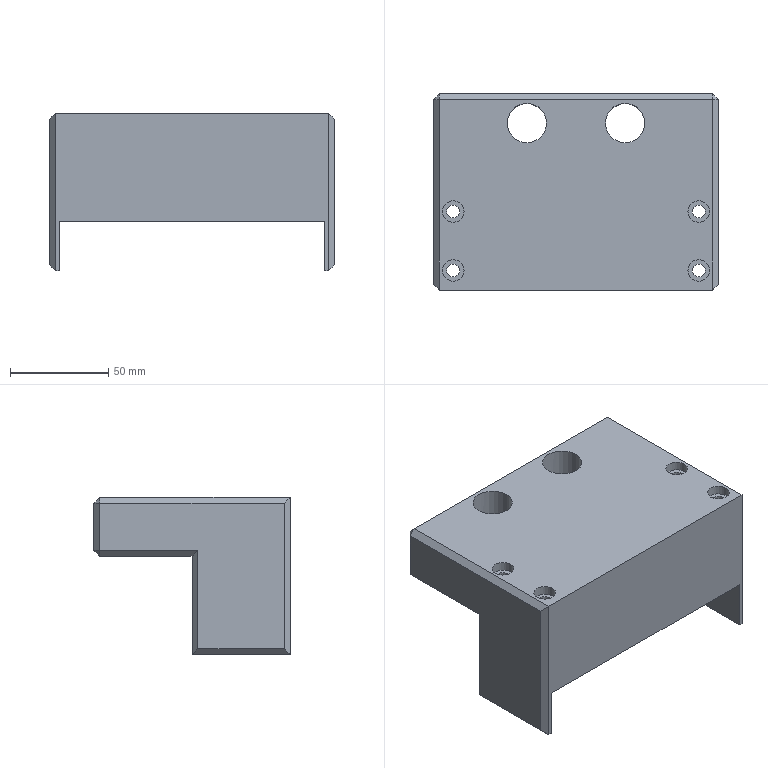Part | 1 solid | 48 faces | box 145 x 100 x 80 mm | volume 596395 mm3 | plane 34 | cylinder 12 | cone 2 | commonest cylinder face diameters 6.6 x4 11 x4 5 x2 20 x2
STEP:
#1=CARTESIAN_POINT('',(72.5,-47.,-3.));
#2=VERTEX_POINT('',#1);
#3=CARTESIAN_POINT('',(72.5,-47.,-77.));
#4=VERTEX_POINT('',#3);
#5=CARTESIAN_POINT('',(72.5,-47.,0.));
#6=DIRECTION('',(0.,0.,-1.));
#7=VECTOR('',#6,1000.);
#8=LINE('',#5,#7);
#9=EDGE_CURVE('',#2,#4,#8,.T.);
#10=ORIENTED_EDGE('',*,*,#9,.T.);
#11=CARTESIAN_POINT('',(72.5,-3.,-77.));
#12=VERTEX_POINT('',#11);
#13=CARTESIAN_POINT('',(72.5,50.,-77.));
#14=DIRECTION('',(0.,1.,0.));
#15=VECTOR('',#14,1000.);
#16=LINE('',#13,#15);
#17=EDGE_CURVE('',#4,#12,#16,.T.);
#18=ORIENTED_EDGE('',*,*,#17,.T.);
#19=CARTESIAN_POINT('',(72.5,-3.,-27.));
#20=VERTEX_POINT('',#19);
#21=CARTESIAN_POINT('',(72.5,-3.,0.));
#22=DIRECTION('',(0.,0.,1.));
#23=VECTOR('',#22,1000.);
#24=LINE('',#21,#23);
#25=EDGE_CURVE('',#12,#20,#24,.T.);
#26=ORIENTED_EDGE('',*,*,#25,.T.);
#27=CARTESIAN_POINT('',(72.5,47.,-27.));
#28=VERTEX_POINT('',#27);
#29=CARTESIAN_POINT('',(72.5,50.,-27.));
#30=DIRECTION('',(0.,1.,0.));
#31=VECTOR('',#30,1000.);
#32=LINE('',#29,#31);
#33=EDGE_CURVE('',#20,#28,#32,.T.);
#34=ORIENTED_EDGE('',*,*,#33,.T.);
#35=CARTESIAN_POINT('',(72.5,47.,-3.));
#36=VERTEX_POINT('',#35);
#37=CARTESIAN_POINT('',(72.5,47.,0.));
#38=DIRECTION('',(0.,0.,1.));
#39=VECTOR('',#38,1000.);
#40=LINE('',#37,#39);
#41=EDGE_CURVE('',#28,#36,#40,.T.);
#42=ORIENTED_EDGE('',*,*,#41,.T.);
#43=CARTESIAN_POINT('',(72.5,-50.,-3.));
#44=DIRECTION('',(0.,-1.,0.));
#45=VECTOR('',#44,1000.);
#46=LINE('',#43,#45);
#47=EDGE_CURVE('',#36,#2,#46,.T.);
#48=ORIENTED_EDGE('',*,*,#47,.T.);
#49=EDGE_LOOP('',(#10,#18,#26,#34,#42,#48));
#50=FACE_BOUND('',#49,.T.);
#51=CARTESIAN_POINT('',(72.5,50.,0.));
#52=DIRECTION('',(-1.,0.,0.));
#53=DIRECTION('',(0.,0.,1.));
#54=AXIS2_PLACEMENT_3D('',#51,#52,#53);
#55=PLANE('',#54);
#56=ADVANCED_FACE('',(#50),#55,.F.);
#57=CARTESIAN_POINT('',(67.5,0.,-80.));
#58=VERTEX_POINT('',#57);
#59=CARTESIAN_POINT('',(69.5,0.,-80.));
#60=VERTEX_POINT('',#59);
#61=CARTESIAN_POINT('',(-72.5,0.,-80.));
#62=DIRECTION('',(1.,0.,0.));
#63=VECTOR('',#62,1000.);
#64=LINE('',#61,#63);
#65=EDGE_CURVE('',#58,#60,#64,.T.);
#66=ORIENTED_EDGE('',*,*,#65,.T.);
#67=CARTESIAN_POINT('',(69.5,-50.,-80.));
#68=VERTEX_POINT('',#67);
#69=CARTESIAN_POINT('',(69.5,50.,-80.));
#70=DIRECTION('',(0.,-1.,0.));
#71=VECTOR('',#70,1000.);
#72=LINE('',#69,#71);
#73=EDGE_CURVE('',#60,#68,#72,.T.);
#74=ORIENTED_EDGE('',*,*,#73,.T.);
#75=CARTESIAN_POINT('',(67.5,-50.,-80.));
#76=VERTEX_POINT('',#75);
#77=CARTESIAN_POINT('',(72.5,-50.,-80.));
#78=DIRECTION('',(-1.,0.,0.));
#79=VECTOR('',#78,1000.);
#80=LINE('',#77,#79);
#81=EDGE_CURVE('',#68,#76,#80,.T.);
#82=ORIENTED_EDGE('',*,*,#81,.T.);
#83=CARTESIAN_POINT('',(67.5,50.,-80.));
#84=DIRECTION('',(0.,-1.,0.));
#85=VECTOR('',#84,1000.);
#86=LINE('',#83,#85);
#87=EDGE_CURVE('',#58,#76,#86,.T.);
#88=ORIENTED_EDGE('',*,*,#87,.F.);
#89=EDGE_LOOP('',(#66,#74,#82,#88));
#90=FACE_BOUND('',#89,.T.);
#91=CARTESIAN_POINT('',(72.5,50.,-80.));
#92=DIRECTION('',(0.,0.,1.));
#93=DIRECTION('',(1.,0.,0.));
#94=AXIS2_PLACEMENT_3D('',#91,#92,#93);
#95=PLANE('',#94);
#96=ADVANCED_FACE('',(#90),#95,.F.);
#97=CARTESIAN_POINT('',(67.5,0.,-55.));
#98=VERTEX_POINT('',#97);
#99=CARTESIAN_POINT('',(67.5,-50.,-55.));
#100=VERTEX_POINT('',#99);
#101=CARTESIAN_POINT('',(67.5,50.,-55.));
#102=DIRECTION('',(0.,-1.,0.));
#103=VECTOR('',#102,1000.);
#104=LINE('',#101,#103);
#105=EDGE_CURVE('',#98,#100,#104,.T.);
#106=ORIENTED_EDGE('',*,*,#105,.F.);
#107=CARTESIAN_POINT('',(67.5,0.,-80.));
#108=DIRECTION('',(0.,0.,-1.));
#109=VECTOR('',#108,1000.);
#110=LINE('',#107,#109);
#111=EDGE_CURVE('',#98,#58,#110,.T.);
#112=ORIENTED_EDGE('',*,*,#111,.T.);
#113=ORIENTED_EDGE('',*,*,#87,.T.);
#114=CARTESIAN_POINT('',(67.5,-50.,-80.));
#115=DIRECTION('',(0.,0.,1.));
#116=VECTOR('',#115,1000.);
#117=LINE('',#114,#116);
#118=EDGE_CURVE('',#76,#100,#117,.T.);
#119=ORIENTED_EDGE('',*,*,#118,.T.);
#120=EDGE_LOOP('',(#106,#112,#113,#119));
#121=FACE_BOUND('',#120,.T.);
#122=CARTESIAN_POINT('',(67.5,50.,-80.));
#123=DIRECTION('',(1.,0.,0.));
#124=DIRECTION('',(0.,0.,-1.));
#125=AXIS2_PLACEMENT_3D('',#122,#123,#124);
#126=PLANE('',#125);
#127=ADVANCED_FACE('',(#121),#126,.F.);
#128=CARTESIAN_POINT('',(-65.8,-10.,-55.));
#129=VERTEX_POINT('',#128);
#130=CARTESIAN_POINT('',(-62.5,-10.,-55.));
#131=DIRECTION('',(0.,0.,-1.));
#132=DIRECTION('',(-1.,0.,0.));
#133=AXIS2_PLACEMENT_3D('',#130,#131,#132);
#134=CIRCLE('',#133,3.3);
#135=EDGE_CURVE('',#129,#129,#134,.T.);
#136=ORIENTED_EDGE('',*,*,#135,.F.);
#137=EDGE_LOOP('',(#136));
#138=FACE_BOUND('',#137,.T.);
#139=CARTESIAN_POINT('',(-65.8,-40.,-55.));
#140=VERTEX_POINT('',#139);
#141=CARTESIAN_POINT('',(-62.5,-40.,-55.));
#142=DIRECTION('',(0.,0.,-1.));
#143=DIRECTION('',(-1.,0.,0.));
#144=AXIS2_PLACEMENT_3D('',#141,#142,#143);
#145=CIRCLE('',#144,3.3);
#146=EDGE_CURVE('',#140,#140,#145,.T.);
#147=ORIENTED_EDGE('',*,*,#146,.F.);
#148=EDGE_LOOP('',(#147));
#149=FACE_BOUND('',#148,.T.);
#150=CARTESIAN_POINT('',(59.2,-10.,-55.));
#151=VERTEX_POINT('',#150);
#152=CARTESIAN_POINT('',(62.5,-10.,-55.));
#153=DIRECTION('',(0.,0.,-1.));
#154=DIRECTION('',(-1.,0.,0.));
#155=AXIS2_PLACEMENT_3D('',#152,#153,#154);
#156=CIRCLE('',#155,3.3);
#157=EDGE_CURVE('',#151,#151,#156,.T.);
#158=ORIENTED_EDGE('',*,*,#157,.F.);
#159=EDGE_LOOP('',(#158));
#160=FACE_BOUND('',#159,.T.);
#161=CARTESIAN_POINT('',(59.2,-40.,-55.));
#162=VERTEX_POINT('',#161);
#163=CARTESIAN_POINT('',(62.5,-40.,-55.));
#164=DIRECTION('',(0.,0.,-1.));
#165=DIRECTION('',(-1.,0.,0.));
#166=AXIS2_PLACEMENT_3D('',#163,#164,#165);
#167=CIRCLE('',#166,3.3);
#168=EDGE_CURVE('',#162,#162,#167,.T.);
#169=ORIENTED_EDGE('',*,*,#168,.F.);
#170=EDGE_LOOP('',(#169));
#171=FACE_BOUND('',#170,.T.);
#172=CARTESIAN_POINT('',(-67.5,0.,-55.));
#173=VERTEX_POINT('',#172);
#174=CARTESIAN_POINT('',(-67.5,0.,-55.));
#175=DIRECTION('',(-1.,0.,0.));
#176=VECTOR('',#175,1000.);
#177=LINE('',#174,#176);
#178=EDGE_CURVE('',#98,#173,#177,.T.);
#179=ORIENTED_EDGE('',*,*,#178,.F.);
#180=ORIENTED_EDGE('',*,*,#105,.T.);
#181=CARTESIAN_POINT('',(-67.5,-50.,-55.));
#182=VERTEX_POINT('',#181);
#183=CARTESIAN_POINT('',(-67.5,-50.,-55.));
#184=DIRECTION('',(1.,0.,0.));
#185=VECTOR('',#184,1000.);
#186=LINE('',#183,#185);
#187=EDGE_CURVE('',#182,#100,#186,.T.);
#188=ORIENTED_EDGE('',*,*,#187,.F.);
#189=CARTESIAN_POINT('',(-67.5,50.,-55.));
#190=DIRECTION('',(0.,-1.,0.));
#191=VECTOR('',#190,1000.);
#192=LINE('',#189,#191);
#193=EDGE_CURVE('',#173,#182,#192,.T.);
#194=ORIENTED_EDGE('',*,*,#193,.F.);
#195=EDGE_LOOP('',(#179,#180,#188,#194));
#196=FACE_BOUND('',#195,.T.);
#197=CARTESIAN_POINT('',(-67.5,50.,-55.));
#198=DIRECTION('',(0.,0.,-1.));
#199=DIRECTION('',(-1.,0.,0.));
#200=AXIS2_PLACEMENT_3D('',#197,#198,#199);
#201=PLANE('',#200);
#202=ADVANCED_FACE('',(#138,#149,#160,#171,#196),#201,.T.);
#203=CARTESIAN_POINT('',(-67.5,0.,-80.));
#204=VERTEX_POINT('',#203);
#205=CARTESIAN_POINT('',(-67.5,0.,-80.));
#206=DIRECTION('',(0.,0.,-1.));
#207=VECTOR('',#206,1000.);
#208=LINE('',#205,#207);
#209=EDGE_CURVE('',#173,#204,#208,.T.);
#210=ORIENTED_EDGE('',*,*,#209,.F.);
#211=ORIENTED_EDGE('',*,*,#193,.T.);
#212=CARTESIAN_POINT('',(-67.5,-50.,-80.));
#213=VERTEX_POINT('',#212);
#214=CARTESIAN_POINT('',(-67.5,-50.,-80.));
#215=DIRECTION('',(0.,0.,1.));
#216=VECTOR('',#215,1000.);
#217=LINE('',#214,#216);
#218=EDGE_CURVE('',#213,#182,#217,.T.);
#219=ORIENTED_EDGE('',*,*,#218,.F.);
#220=CARTESIAN_POINT('',(-67.5,50.,-80.));
#221=DIRECTION('',(0.,-1.,0.));
#222=VECTOR('',#221,1000.);
#223=LINE('',#220,#222);
#224=EDGE_CURVE('',#204,#213,#223,.T.);
#225=ORIENTED_EDGE('',*,*,#224,.F.);
#226=EDGE_LOOP('',(#210,#211,#219,#225));
#227=FACE_BOUND('',#226,.T.);
#228=CARTESIAN_POINT('',(-67.5,50.,-80.));
#229=DIRECTION('',(1.,0.,0.));
#230=DIRECTION('',(0.,0.,-1.));
#231=AXIS2_PLACEMENT_3D('',#228,#229,#230);
#232=PLANE('',#231);
#233=ADVANCED_FACE('',(#227),#232,.T.);
#234=CARTESIAN_POINT('',(-69.5,-50.,-80.));
#235=VERTEX_POINT('',#234);
#236=CARTESIAN_POINT('',(-67.5,-50.,-80.));
#237=DIRECTION('',(-1.,0.,0.));
#238=VECTOR('',#237,1000.);
#239=LINE('',#236,#238);
#240=EDGE_CURVE('',#213,#235,#239,.T.);
#241=ORIENTED_EDGE('',*,*,#240,.T.);
#242=CARTESIAN_POINT('',(-69.5,0.,-80.));
#243=VERTEX_POINT('',#242);
#244=CARTESIAN_POINT('',(-69.5,0.,-80.));
#245=DIRECTION('',(0.,1.,0.));
#246=VECTOR('',#245,1000.);
#247=LINE('',#244,#246);
#248=EDGE_CURVE('',#235,#243,#247,.T.);
#249=ORIENTED_EDGE('',*,*,#248,.T.);
#250=CARTESIAN_POINT('',(-72.5,0.,-80.));
#251=DIRECTION('',(1.,0.,0.));
#252=VECTOR('',#251,1000.);
#253=LINE('',#250,#252);
#254=EDGE_CURVE('',#243,#204,#253,.T.);
#255=ORIENTED_EDGE('',*,*,#254,.T.);
#256=ORIENTED_EDGE('',*,*,#224,.T.);
#257=EDGE_LOOP('',(#241,#249,#255,#256));
#258=FACE_BOUND('',#257,.T.);
#259=CARTESIAN_POINT('',(-67.5,50.,-80.));
#260=DIRECTION('',(0.,0.,1.));
#261=DIRECTION('',(1.,0.,0.));
#262=AXIS2_PLACEMENT_3D('',#259,#260,#261);
#263=PLANE('',#262);
#264=ADVANCED_FACE('',(#258),#263,.F.);
#265=CARTESIAN_POINT('',(-72.5,-47.,-77.));
#266=VERTEX_POINT('',#265);
#267=CARTESIAN_POINT('',(-72.5,-47.,-3.));
#268=VERTEX_POINT('',#267);
#269=CARTESIAN_POINT('',(-72.5,-47.,0.));
#270=DIRECTION('',(0.,0.,1.));
#271=VECTOR('',#270,1000.);
#272=LINE('',#269,#271);
#273=EDGE_CURVE('',#266,#268,#272,.T.);
#274=ORIENTED_EDGE('',*,*,#273,.T.);
#275=CARTESIAN_POINT('',(-72.5,47.,-3.));
#276=VERTEX_POINT('',#275);
#277=CARTESIAN_POINT('',(-72.5,50.,-3.));
#278=DIRECTION('',(0.,1.,0.));
#279=VECTOR('',#278,1000.);
#280=LINE('',#277,#279);
#281=EDGE_CURVE('',#268,#276,#280,.T.);
#282=ORIENTED_EDGE('',*,*,#281,.T.);
#283=CARTESIAN_POINT('',(-72.5,47.,-27.));
#284=VERTEX_POINT('',#283);
#285=CARTESIAN_POINT('',(-72.5,47.,0.));
#286=DIRECTION('',(0.,0.,-1.));
#287=VECTOR('',#286,1000.);
#288=LINE('',#285,#287);
#289=EDGE_CURVE('',#276,#284,#288,.T.);
#290=ORIENTED_EDGE('',*,*,#289,.T.);
#291=CARTESIAN_POINT('',(-72.5,-3.,-27.));
#292=VERTEX_POINT('',#291);
#293=CARTESIAN_POINT('',(-72.5,0.,-27.));
#294=DIRECTION('',(0.,-1.,0.));
#295=VECTOR('',#294,1000.);
#296=LINE('',#293,#295);
#297=EDGE_CURVE('',#284,#292,#296,.T.);
#298=ORIENTED_EDGE('',*,*,#297,.T.);
#299=CARTESIAN_POINT('',(-72.5,-3.,-77.));
#300=VERTEX_POINT('',#299);
#301=CARTESIAN_POINT('',(-72.5,-3.,-80.));
#302=DIRECTION('',(0.,0.,-1.));
#303=VECTOR('',#302,1000.);
#304=LINE('',#301,#303);
#305=EDGE_CURVE('',#292,#300,#304,.T.);
#306=ORIENTED_EDGE('',*,*,#305,.T.);
#307=CARTESIAN_POINT('',(-72.5,-50.,-77.));
#308=DIRECTION('',(0.,-1.,0.));
#309=VECTOR('',#308,1000.);
#310=LINE('',#307,#309);
#311=EDGE_CURVE('',#300,#266,#310,.T.);
#312=ORIENTED_EDGE('',*,*,#311,.T.);
#313=EDGE_LOOP('',(#274,#282,#290,#298,#306,#312));
#314=FACE_BOUND('',#313,.T.);
#315=CARTESIAN_POINT('',(-72.5,50.,0.));
#316=DIRECTION('',(-1.,0.,0.));
#317=DIRECTION('',(0.,0.,1.));
#318=AXIS2_PLACEMENT_3D('',#315,#316,#317);
#319=PLANE('',#318);
#320=ADVANCED_FACE('',(#314),#319,.T.);
#321=CARTESIAN_POINT('',(69.5,-50.,0.));
#322=VERTEX_POINT('',#321);
#323=CARTESIAN_POINT('',(-69.5,-50.,0.));
#324=VERTEX_POINT('',#323);
#325=CARTESIAN_POINT('',(72.5,-50.,0.));
#326=DIRECTION('',(-1.,0.,0.));
#327=VECTOR('',#326,1000.);
#328=LINE('',#325,#327);
#329=EDGE_CURVE('',#322,#324,#328,.T.);
#330=ORIENTED_EDGE('',*,*,#329,.F.);
#331=CARTESIAN_POINT('',(69.5,47.,0.));
#332=VERTEX_POINT('',#331);
#333=CARTESIAN_POINT('',(69.5,50.,0.));
#334=DIRECTION('',(0.,1.,0.));
#335=VECTOR('',#334,1000.);
#336=LINE('',#333,#335);
#337=EDGE_CURVE('',#322,#332,#336,.T.);
#338=ORIENTED_EDGE('',*,*,#337,.T.);
#339=CARTESIAN_POINT('',(-69.5,47.,0.));
#340=VERTEX_POINT('',#339);
#341=CARTESIAN_POINT('',(72.5,47.,0.));
#342=DIRECTION('',(-1.,0.,0.));
#343=VECTOR('',#342,1000.);
#344=LINE('',#341,#343);
#345=EDGE_CURVE('',#332,#340,#344,.T.);
#346=ORIENTED_EDGE('',*,*,#345,.T.);
#347=CARTESIAN_POINT('',(-69.5,50.,0.));
#348=DIRECTION('',(0.,-1.,0.));
#349=VECTOR('',#348,1000.);
#350=LINE('',#347,#349);
#351=EDGE_CURVE('',#340,#324,#350,.T.);
#352=ORIENTED_EDGE('',*,*,#351,.T.);
#353=EDGE_LOOP('',(#330,#338,#346,#352));
#354=FACE_BOUND('',#353,.T.);
#355=CARTESIAN_POINT('',(35.,35.,0.));
#356=VERTEX_POINT('',#355);
#357=CARTESIAN_POINT('',(25.,35.,0.));
#358=DIRECTION('',(0.,0.,1.));
#359=DIRECTION('',(1.,0.,0.));
#360=AXIS2_PLACEMENT_3D('',#357,#358,#359);
#361=CIRCLE('',#360,10.);
#362=EDGE_CURVE('',#356,#356,#361,.T.);
#363=ORIENTED_EDGE('',*,*,#362,.F.);
#364=EDGE_LOOP('',(#363));
#365=FACE_BOUND('',#364,.T.);
#366=CARTESIAN_POINT('',(-15.,35.,0.));
#367=VERTEX_POINT('',#366);
#368=CARTESIAN_POINT('',(-25.,35.,0.));
#369=DIRECTION('',(0.,0.,1.));
#370=DIRECTION('',(1.,0.,0.));
#371=AXIS2_PLACEMENT_3D('',#368,#369,#370);
#372=CIRCLE('',#371,10.);
#373=EDGE_CURVE('',#367,#367,#372,.T.);
#374=ORIENTED_EDGE('',*,*,#373,.F.);
#375=EDGE_LOOP('',(#374));
#376=FACE_BOUND('',#375,.T.);
#377=CARTESIAN_POINT('',(-57.,-10.,0.));
#378=VERTEX_POINT('',#377);
#379=CARTESIAN_POINT('',(-62.5,-10.,0.));
#380=DIRECTION('',(0.,0.,1.));
#381=DIRECTION('',(1.,0.,0.));
#382=AXIS2_PLACEMENT_3D('',#379,#380,#381);
#383=CIRCLE('',#382,5.5);
#384=EDGE_CURVE('',#378,#378,#383,.T.);
#385=ORIENTED_EDGE('',*,*,#384,.F.);
#386=EDGE_LOOP('',(#385));
#387=FACE_BOUND('',#386,.T.);
#388=CARTESIAN_POINT('',(-57.,-40.,0.));
#389=VERTEX_POINT('',#388);
#390=CARTESIAN_POINT('',(-62.5,-40.,0.));
#391=DIRECTION('',(0.,0.,1.));
#392=DIRECTION('',(1.,0.,0.));
#393=AXIS2_PLACEMENT_3D('',#390,#391,#392);
#394=CIRCLE('',#393,5.5);
#395=EDGE_CURVE('',#389,#389,#394,.T.);
#396=ORIENTED_EDGE('',*,*,#395,.F.);
#397=EDGE_LOOP('',(#396));
#398=FACE_BOUND('',#397,.T.);
#399=CARTESIAN_POINT('',(68.,-10.,0.));
#400=VERTEX_POINT('',#399);
#401=CARTESIAN_POINT('',(62.5,-10.,0.));
#402=DIRECTION('',(0.,0.,1.));
#403=DIRECTION('',(1.,0.,0.));
#404=AXIS2_PLACEMENT_3D('',#401,#402,#403);
#405=CIRCLE('',#404,5.5);
#406=EDGE_CURVE('',#400,#400,#405,.T.);
#407=ORIENTED_EDGE('',*,*,#406,.F.);
#408=EDGE_LOOP('',(#407));
#409=FACE_BOUND('',#408,.T.);
#410=CARTESIAN_POINT('',(68.,-40.,0.));
#411=VERTEX_POINT('',#410);
#412=CARTESIAN_POINT('',(62.5,-40.,0.));
#413=DIRECTION('',(0.,0.,1.));
#414=DIRECTION('',(1.,0.,0.));
#415=AXIS2_PLACEMENT_3D('',#412,#413,#414);
#416=CIRCLE('',#415,5.5);
#417=EDGE_CURVE('',#411,#411,#416,.T.);
#418=ORIENTED_EDGE('',*,*,#417,.F.);
#419=EDGE_LOOP('',(#418));
#420=FACE_BOUND('',#419,.T.);
#421=CARTESIAN_POINT('',(72.5,50.,0.));
#422=DIRECTION('',(0.,0.,1.));
#423=DIRECTION('',(1.,0.,0.));
#424=AXIS2_PLACEMENT_3D('',#421,#422,#423);
#425=PLANE('',#424);
#426=ADVANCED_FACE('',(#354,#365,#376,#387,#398,#409,#420),#425,.T.);
#427=CARTESIAN_POINT('',(-69.5,50.,-3.));
#428=VERTEX_POINT('',#427);
#429=CARTESIAN_POINT('',(69.5,50.,-3.));
#430=VERTEX_POINT('',#429);
#431=CARTESIAN_POINT('',(72.5,50.,-3.));
#432=DIRECTION('',(1.,0.,0.));
#433=VECTOR('',#432,1000.);
#434=LINE('',#431,#433);
#435=EDGE_CURVE('',#428,#430,#434,.T.);
#436=ORIENTED_EDGE('',*,*,#435,.T.);
#437=CARTESIAN_POINT('',(69.5,50.,-27.));
#438=VERTEX_POINT('',#437);
#439=CARTESIAN_POINT('',(69.5,50.,-30.));
#440=DIRECTION('',(0.,0.,-1.));
#441=VECTOR('',#440,1000.);
#442=LINE('',#439,#441);
#443=EDGE_CURVE('',#430,#438,#442,.T.);
#444=ORIENTED_EDGE('',*,*,#443,.T.);
#445=CARTESIAN_POINT('',(-69.5,50.,-27.));
#446=VERTEX_POINT('',#445);
#447=CARTESIAN_POINT('',(-72.5,50.,-27.));
#448=DIRECTION('',(-1.,0.,0.));
#449=VECTOR('',#448,1000.);
#450=LINE('',#447,#449);
#451=EDGE_CURVE('',#438,#446,#450,.T.);
#452=ORIENTED_EDGE('',*,*,#451,.T.);
#453=CARTESIAN_POINT('',(-69.5,50.,0.));
#454=DIRECTION('',(0.,0.,1.));
#455=VECTOR('',#454,1000.);
#456=LINE('',#453,#455);
#457=EDGE_CURVE('',#446,#428,#456,.T.);
#458=ORIENTED_EDGE('',*,*,#457,.T.);
#459=EDGE_LOOP('',(#436,#444,#452,#458));
#460=FACE_BOUND('',#459,.T.);
#461=CARTESIAN_POINT('',(25.,50.,-9.5));
#462=VERTEX_POINT('',#461);
#463=CARTESIAN_POINT('',(25.,50.,-15.));
#464=DIRECTION('',(0.,1.,0.));
#465=DIRECTION('',(0.,0.,1.));
#466=AXIS2_PLACEMENT_3D('',#463,#464,#465);
#467=CIRCLE('',#466,5.5);
#468=EDGE_CURVE('',#462,#462,#467,.F.);
#469=ORIENTED_EDGE('',*,*,#468,.T.);
#470=EDGE_LOOP('',(#469));
#471=FACE_BOUND('',#470,.T.);
#472=CARTESIAN_POINT('',(-25.,50.,-9.5));
#473=VERTEX_POINT('',#472);
#474=CARTESIAN_POINT('',(-25.,50.,-15.));
#475=DIRECTION('',(0.,1.,0.));
#476=DIRECTION('',(0.,0.,1.));
#477=AXIS2_PLACEMENT_3D('',#474,#475,#476);
#478=CIRCLE('',#477,5.5);
#479=EDGE_CURVE('',#473,#473,#478,.F.);
#480=ORIENTED_EDGE('',*,*,#479,.T.);
#481=EDGE_LOOP('',(#480));
#482=FACE_BOUND('',#481,.T.);
#483=CARTESIAN_POINT('',(72.5,50.,0.));
#484=DIRECTION('',(0.,1.,0.));
#485=DIRECTION('',(0.,0.,1.));
#486=AXIS2_PLACEMENT_3D('',#483,#484,#485);
#487=PLANE('',#486);
#488=ADVANCED_FACE('',(#460,#471,#482),#487,.T.);
#489=ORIENTED_EDGE('',*,*,#81,.F.);
#490=CARTESIAN_POINT('',(69.5,-50.,0.));
#491=DIRECTION('',(0.,0.,1.));
#492=VECTOR('',#491,1000.);
#493=LINE('',#490,#492);
#494=EDGE_CURVE('',#68,#322,#493,.T.);
#495=ORIENTED_EDGE('',*,*,#494,.T.);
#496=ORIENTED_EDGE('',*,*,#329,.T.);
#497=CARTESIAN_POINT('',(-69.5,-50.,-80.));
#498=DIRECTION('',(0.,0.,-1.));
#499=VECTOR('',#498,1000.);
#500=LINE('',#497,#499);
#501=EDGE_CURVE('',#324,#235,#500,.T.);
#502=ORIENTED_EDGE('',*,*,#501,.T.);
#503=ORIENTED_EDGE('',*,*,#240,.F.);
#504=ORIENTED_EDGE('',*,*,#218,.T.);
#505=ORIENTED_EDGE('',*,*,#187,.T.);
#506=ORIENTED_EDGE('',*,*,#118,.F.);
#507=EDGE_LOOP('',(#489,#495,#496,#502,#503,#504,#505,#506));
#508=FACE_BOUND('',#507,.T.);
#509=CARTESIAN_POINT('',(72.5,-50.,0.));
#510=DIRECTION('',(0.,1.,0.));
#511=DIRECTION('',(0.,0.,1.));
#512=AXIS2_PLACEMENT_3D('',#509,#510,#511);
#513=PLANE('',#512);
#514=ADVANCED_FACE('',(#508),#513,.F.);
#515=CARTESIAN_POINT('',(-69.5,0.,-30.));
#516=VERTEX_POINT('',#515);
#517=CARTESIAN_POINT('',(69.5,0.,-30.));
#518=VERTEX_POINT('',#517);
#519=CARTESIAN_POINT('',(-72.5,0.,-30.));
#520=DIRECTION('',(1.,0.,0.));
#521=VECTOR('',#520,1000.);
#522=LINE('',#519,#521);
#523=EDGE_CURVE('',#516,#518,#522,.T.);
#524=ORIENTED_EDGE('',*,*,#523,.T.);
#525=CARTESIAN_POINT('',(69.5,0.,0.));
#526=DIRECTION('',(0.,0.,-1.));
#527=VECTOR('',#526,1000.);
#528=LINE('',#525,#527);
#529=EDGE_CURVE('',#518,#60,#528,.T.);
#530=ORIENTED_EDGE('',*,*,#529,.T.);
#531=ORIENTED_EDGE('',*,*,#65,.F.);
#532=ORIENTED_EDGE('',*,*,#111,.F.);
#533=ORIENTED_EDGE('',*,*,#178,.T.);
#534=ORIENTED_EDGE('',*,*,#209,.T.);
#535=ORIENTED_EDGE('',*,*,#254,.F.);
#536=CARTESIAN_POINT('',(-69.5,0.,-30.));
#537=DIRECTION('',(0.,0.,1.));
#538=VECTOR('',#537,1000.);
#539=LINE('',#536,#538);
#540=EDGE_CURVE('',#243,#516,#539,.T.);
#541=ORIENTED_EDGE('',*,*,#540,.T.);
#542=EDGE_LOOP('',(#524,#530,#531,#532,#533,#534,#535,#541));
#543=FACE_BOUND('',#542,.T.);
#544=CARTESIAN_POINT('',(72.5,0.,0.));
#545=DIRECTION('',(0.,-1.,0.));
#546=DIRECTION('',(0.,0.,-1.));
#547=AXIS2_PLACEMENT_3D('',#544,#545,#546);
#548=PLANE('',#547);
#549=ADVANCED_FACE('',(#543),#548,.F.);
#550=CARTESIAN_POINT('',(35.,35.,-30.));
#551=VERTEX_POINT('',#550);
#552=CARTESIAN_POINT('',(25.,35.,-30.));
#553=DIRECTION('',(0.,0.,1.));
#554=DIRECTION('',(1.,0.,0.));
#555=AXIS2_PLACEMENT_3D('',#552,#553,#554);
#556=CIRCLE('',#555,10.);
#557=EDGE_CURVE('',#551,#551,#556,.T.);
#558=ORIENTED_EDGE('',*,*,#557,.T.);
#559=EDGE_LOOP('',(#558));
#560=FACE_BOUND('',#559,.T.);
#561=CARTESIAN_POINT('',(-15.,35.,-30.));
#562=VERTEX_POINT('',#561);
#563=CARTESIAN_POINT('',(-25.,35.,-30.));
#564=DIRECTION('',(0.,0.,1.));
#565=DIRECTION('',(1.,0.,0.));
#566=AXIS2_PLACEMENT_3D('',#563,#564,#565);
#567=CIRCLE('',#566,10.);
#568=EDGE_CURVE('',#562,#562,#567,.T.);
#569=ORIENTED_EDGE('',*,*,#568,.T.);
#570=EDGE_LOOP('',(#569));
#571=FACE_BOUND('',#570,.T.);
#572=CARTESIAN_POINT('',(-69.5,47.,-30.));
#573=VERTEX_POINT('',#572);
#574=CARTESIAN_POINT('',(69.5,47.,-30.));
#575=VERTEX_POINT('',#574);
#576=CARTESIAN_POINT('',(72.5,47.,-30.));
#577=DIRECTION('',(1.,0.,0.));
#578=VECTOR('',#577,1000.);
#579=LINE('',#576,#578);
#580=EDGE_CURVE('',#573,#575,#579,.T.);
#581=ORIENTED_EDGE('',*,*,#580,.T.);
#582=CARTESIAN_POINT('',(69.5,0.,-30.));
#583=DIRECTION('',(0.,-1.,0.));
#584=VECTOR('',#583,1000.);
#585=LINE('',#582,#584);
#586=EDGE_CURVE('',#575,#518,#585,.T.);
#587=ORIENTED_EDGE('',*,*,#586,.T.);
#588=ORIENTED_EDGE('',*,*,#523,.F.);
#589=CARTESIAN_POINT('',(-69.5,50.,-30.));
#590=DIRECTION('',(0.,1.,0.));
#591=VECTOR('',#590,1000.);
#592=LINE('',#589,#591);
#593=EDGE_CURVE('',#516,#573,#592,.T.);
#594=ORIENTED_EDGE('',*,*,#593,.T.);
#595=EDGE_LOOP('',(#581,#587,#588,#594));
#596=FACE_BOUND('',#595,.T.);
#597=CARTESIAN_POINT('',(-72.5,0.,-30.));
#598=DIRECTION('',(0.,0.,1.));
#599=DIRECTION('',(1.,0.,0.));
#600=AXIS2_PLACEMENT_3D('',#597,#598,#599);
#601=PLANE('',#600);
#602=ADVANCED_FACE('',(#560,#571,#596),#601,.F.);
#603=ORIENTED_EDGE('',*,*,#168,.T.);
#604=EDGE_LOOP('',(#603));
#605=FACE_BOUND('',#604,.T.);
#606=CARTESIAN_POINT('',(65.8,-40.,-4.7));
#607=VERTEX_POINT('',#606);
#608=CARTESIAN_POINT('',(62.5,-40.,-4.7));
#609=DIRECTION('',(0.,0.,1.));
#610=DIRECTION('',(1.,0.,0.));
#611=AXIS2_PLACEMENT_3D('',#608,#609,#610);
#612=CIRCLE('',#611,3.3);
#613=EDGE_CURVE('',#607,#607,#612,.T.);
#614=ORIENTED_EDGE('',*,*,#613,.T.);
#615=EDGE_LOOP('',(#614));
#616=FACE_BOUND('',#615,.T.);
#617=CARTESIAN_POINT('',(62.5,-40.,0.));
#618=DIRECTION('',(0.,0.,1.));
#619=DIRECTION('',(1.,0.,0.));
#620=AXIS2_PLACEMENT_3D('',#617,#618,#619);
#621=CYLINDRICAL_SURFACE('',#620,3.3);
#622=ADVANCED_FACE('',(#605,#616),#621,.F.);
#623=ORIENTED_EDGE('',*,*,#613,.F.);
#624=EDGE_LOOP('',(#623));
#625=FACE_BOUND('',#624,.T.);
#626=CARTESIAN_POINT('',(68.,-40.,-4.7));
#627=VERTEX_POINT('',#626);
#628=CARTESIAN_POINT('',(62.5,-40.,-4.7));
#629=DIRECTION('',(0.,0.,1.));
#630=DIRECTION('',(1.,0.,0.));
#631=AXIS2_PLACEMENT_3D('',#628,#629,#630);
#632=CIRCLE('',#631,5.5);
#633=EDGE_CURVE('',#627,#627,#632,.T.);
#634=ORIENTED_EDGE('',*,*,#633,.T.);
#635=EDGE_LOOP('',(#634));
#636=FACE_BOUND('',#635,.T.);
#637=CARTESIAN_POINT('',(65.8,-40.,-4.7));
#638=DIRECTION('',(0.,0.,-1.));
#639=DIRECTION('',(-1.,0.,0.));
#640=AXIS2_PLACEMENT_3D('',#637,#638,#639);
#641=PLANE('',#640);
#642=ADVANCED_FACE('',(#625,#636),#641,.F.);
#643=ORIENTED_EDGE('',*,*,#633,.F.);
#644=EDGE_LOOP('',(#643));
#645=FACE_BOUND('',#644,.T.);
#646=ORIENTED_EDGE('',*,*,#417,.T.);
#647=EDGE_LOOP('',(#646));
#648=FACE_BOUND('',#647,.T.);
#649=CARTESIAN_POINT('',(62.5,-40.,0.));
#650=DIRECTION('',(0.,0.,1.));
#651=DIRECTION('',(1.,0.,0.));
#652=AXIS2_PLACEMENT_3D('',#649,#650,#651);
#653=CYLINDRICAL_SURFACE('',#652,5.5);
#654=ADVANCED_FACE('',(#645,#648),#653,.F.);
#655=ORIENTED_EDGE('',*,*,#157,.T.);
#656=EDGE_LOOP('',(#655));
#657=FACE_BOUND('',#656,.T.);
#658=CARTESIAN_POINT('',(65.8,-10.,-4.7));
#659=VERTEX_POINT('',#658);
#660=CARTESIAN_POINT('',(62.5,-10.,-4.7));
#661=DIRECTION('',(0.,0.,1.));
#662=DIRECTION('',(1.,0.,0.));
#663=AXIS2_PLACEMENT_3D('',#660,#661,#662);
#664=CIRCLE('',#663,3.3);
#665=EDGE_CURVE('',#659,#659,#664,.T.);
#666=ORIENTED_EDGE('',*,*,#665,.T.);
#667=EDGE_LOOP('',(#666));
#668=FACE_BOUND('',#667,.T.);
#669=CARTESIAN_POINT('',(62.5,-10.,0.));
#670=DIRECTION('',(0.,0.,1.));
#671=DIRECTION('',(1.,0.,0.));
#672=AXIS2_PLACEMENT_3D('',#669,#670,#671);
#673=CYLINDRICAL_SURFACE('',#672,3.3);
#674=ADVANCED_FACE('',(#657,#668),#673,.F.);
#675=ORIENTED_EDGE('',*,*,#665,.F.);
#676=EDGE_LOOP('',(#675));
#677=FACE_BOUND('',#676,.T.);
#678=CARTESIAN_POINT('',(68.,-10.,-4.7));
#679=VERTEX_POINT('',#678);
#680=CARTESIAN_POINT('',(62.5,-10.,-4.7));
#681=DIRECTION('',(0.,0.,1.));
#682=DIRECTION('',(1.,0.,0.));
#683=AXIS2_PLACEMENT_3D('',#680,#681,#682);
#684=CIRCLE('',#683,5.5);
#685=EDGE_CURVE('',#679,#679,#684,.T.);
#686=ORIENTED_EDGE('',*,*,#685,.T.);
#687=EDGE_LOOP('',(#686));
#688=FACE_BOUND('',#687,.T.);
#689=CARTESIAN_POINT('',(65.8,-10.,-4.7));
#690=DIRECTION('',(0.,0.,-1.));
#691=DIRECTION('',(-1.,0.,0.));
#692=AXIS2_PLACEMENT_3D('',#689,#690,#691);
#693=PLANE('',#692);
#694=ADVANCED_FACE('',(#677,#688),#693,.F.);
#695=ORIENTED_EDGE('',*,*,#685,.F.);
#696=EDGE_LOOP('',(#695));
#697=FACE_BOUND('',#696,.T.);
#698=ORIENTED_EDGE('',*,*,#406,.T.);
#699=EDGE_LOOP('',(#698));
#700=FACE_BOUND('',#699,.T.);
#701=CARTESIAN_POINT('',(62.5,-10.,0.));
#702=DIRECTION('',(0.,0.,1.));
#703=DIRECTION('',(1.,0.,0.));
#704=AXIS2_PLACEMENT_3D('',#701,#702,#703);
#705=CYLINDRICAL_SURFACE('',#704,5.5);
#706=ADVANCED_FACE('',(#697,#700),#705,.F.);
#707=ORIENTED_EDGE('',*,*,#146,.T.);
#708=EDGE_LOOP('',(#707));
#709=FACE_BOUND('',#708,.T.);
#710=CARTESIAN_POINT('',(-59.2,-40.,-4.7));
#711=VERTEX_POINT('',#710);
#712=CARTESIAN_POINT('',(-62.5,-40.,-4.7));
#713=DIRECTION('',(0.,0.,1.));
#714=DIRECTION('',(1.,0.,0.));
#715=AXIS2_PLACEMENT_3D('',#712,#713,#714);
#716=CIRCLE('',#715,3.3);
#717=EDGE_CURVE('',#711,#711,#716,.T.);
#718=ORIENTED_EDGE('',*,*,#717,.T.);
#719=EDGE_LOOP('',(#718));
#720=FACE_BOUND('',#719,.T.);
#721=CARTESIAN_POINT('',(-62.5,-40.,0.));
#722=DIRECTION('',(0.,0.,1.));
#723=DIRECTION('',(1.,0.,0.));
#724=AXIS2_PLACEMENT_3D('',#721,#722,#723);
#725=CYLINDRICAL_SURFACE('',#724,3.3);
#726=ADVANCED_FACE('',(#709,#720),#725,.F.);
#727=ORIENTED_EDGE('',*,*,#717,.F.);
#728=EDGE_LOOP('',(#727));
#729=FACE_BOUND('',#728,.T.);
#730=CARTESIAN_POINT('',(-57.,-40.,-4.7));
#731=VERTEX_POINT('',#730);
#732=CARTESIAN_POINT('',(-62.5,-40.,-4.7));
#733=DIRECTION('',(0.,0.,1.));
#734=DIRECTION('',(1.,0.,0.));
#735=AXIS2_PLACEMENT_3D('',#732,#733,#734);
#736=CIRCLE('',#735,5.5);
#737=EDGE_CURVE('',#731,#731,#736,.T.);
#738=ORIENTED_EDGE('',*,*,#737,.T.);
#739=EDGE_LOOP('',(#738));
#740=FACE_BOUND('',#739,.T.);
#741=CARTESIAN_POINT('',(-59.2,-40.,-4.7));
#742=DIRECTION('',(0.,0.,-1.));
#743=DIRECTION('',(-1.,0.,0.));
#744=AXIS2_PLACEMENT_3D('',#741,#742,#743);
#745=PLANE('',#744);
#746=ADVANCED_FACE('',(#729,#740),#745,.F.);
#747=ORIENTED_EDGE('',*,*,#737,.F.);
#748=EDGE_LOOP('',(#747));
#749=FACE_BOUND('',#748,.T.);
#750=ORIENTED_EDGE('',*,*,#395,.T.);
#751=EDGE_LOOP('',(#750));
#752=FACE_BOUND('',#751,.T.);
#753=CARTESIAN_POINT('',(-62.5,-40.,0.));
#754=DIRECTION('',(0.,0.,1.));
#755=DIRECTION('',(1.,0.,0.));
#756=AXIS2_PLACEMENT_3D('',#753,#754,#755);
#757=CYLINDRICAL_SURFACE('',#756,5.5);
#758=ADVANCED_FACE('',(#749,#752),#757,.F.);
#759=ORIENTED_EDGE('',*,*,#135,.T.);
#760=EDGE_LOOP('',(#759));
#761=FACE_BOUND('',#760,.T.);
#762=CARTESIAN_POINT('',(-59.2,-10.,-4.7));
#763=VERTEX_POINT('',#762);
#764=CARTESIAN_POINT('',(-62.5,-10.,-4.7));
#765=DIRECTION('',(0.,0.,1.));
#766=DIRECTION('',(1.,0.,0.));
#767=AXIS2_PLACEMENT_3D('',#764,#765,#766);
#768=CIRCLE('',#767,3.3);
#769=EDGE_CURVE('',#763,#763,#768,.T.);
#770=ORIENTED_EDGE('',*,*,#769,.T.);
#771=EDGE_LOOP('',(#770));
#772=FACE_BOUND('',#771,.T.);
#773=CARTESIAN_POINT('',(-62.5,-10.,0.));
#774=DIRECTION('',(0.,0.,1.));
#775=DIRECTION('',(1.,0.,0.));
#776=AXIS2_PLACEMENT_3D('',#773,#774,#775);
#777=CYLINDRICAL_SURFACE('',#776,3.3);
#778=ADVANCED_FACE('',(#761,#772),#777,.F.);
#779=ORIENTED_EDGE('',*,*,#769,.F.);
#780=EDGE_LOOP('',(#779));
#781=FACE_BOUND('',#780,.T.);
#782=CARTESIAN_POINT('',(-57.,-10.,-4.7));
#783=VERTEX_POINT('',#782);
#784=CARTESIAN_POINT('',(-62.5,-10.,-4.7));
#785=DIRECTION('',(0.,0.,1.));
#786=DIRECTION('',(1.,0.,0.));
#787=AXIS2_PLACEMENT_3D('',#784,#785,#786);
#788=CIRCLE('',#787,5.5);
#789=EDGE_CURVE('',#783,#783,#788,.T.);
#790=ORIENTED_EDGE('',*,*,#789,.T.);
#791=EDGE_LOOP('',(#790));
#792=FACE_BOUND('',#791,.T.);
#793=CARTESIAN_POINT('',(-59.2,-10.,-4.7));
#794=DIRECTION('',(0.,0.,-1.));
#795=DIRECTION('',(-1.,0.,0.));
#796=AXIS2_PLACEMENT_3D('',#793,#794,#795);
#797=PLANE('',#796);
#798=ADVANCED_FACE('',(#781,#792),#797,.F.);
#799=ORIENTED_EDGE('',*,*,#789,.F.);
#800=EDGE_LOOP('',(#799));
#801=FACE_BOUND('',#800,.T.);
#802=ORIENTED_EDGE('',*,*,#384,.T.);
#803=EDGE_LOOP('',(#802));
#804=FACE_BOUND('',#803,.T.);
#805=CARTESIAN_POINT('',(-62.5,-10.,0.));
#806=DIRECTION('',(0.,0.,1.));
#807=DIRECTION('',(1.,0.,0.));
#808=AXIS2_PLACEMENT_3D('',#805,#806,#807);
#809=CYLINDRICAL_SURFACE('',#808,5.5);
#810=ADVANCED_FACE('',(#801,#804),#809,.F.);
#811=CARTESIAN_POINT('',(-25.,45.,-12.5));
#812=VERTEX_POINT('',#811);
#813=CARTESIAN_POINT('',(-26.961,44.843,-13.043));
#814=CARTESIAN_POINT('',(-25.,45.078,-12.229));
#815=CARTESIAN_POINT('',(-23.041,44.844,-13.042));
#816=CARTESIAN_POINT('',(-22.23,44.602,-14.997));
#817=CARTESIAN_POINT('',(-23.041,44.844,-16.96));
#818=CARTESIAN_POINT('',(-24.999,45.078,-17.77));
#819=CARTESIAN_POINT('',(-26.957,44.844,-16.961));
#820=CARTESIAN_POINT('',(-27.77,44.602,-15.001));
#821=CARTESIAN_POINT('',(-26.961,44.843,-13.043));
#822=CARTESIAN_POINT('',(-25.,45.078,-12.229));
#823=CARTESIAN_POINT('',(-23.041,44.844,-13.042));
#824=B_SPLINE_CURVE_WITH_KNOTS('',3,(#813,#814,#815,#816,#817,#818,#819,#820,#821,#822,#823),.UNSPECIFIED.,.T.,.F.,(1,1,1,1,1,1,1,1,1,1,1,1,1,1,1),(-0.005885,-0.003923,-0.001962,0.,0.001962,0.003923,0.005885,0.007846,0.009808,0.01177,0.01373,0.01569,0.01765,0.01962,0.02158),.UNSPECIFIED.);
#825=EDGE_CURVE('',#812,#812,#824,.T.);
#826=ORIENTED_EDGE('',*,*,#825,.T.);
#827=EDGE_LOOP('',(#826));
#828=FACE_BOUND('',#827,.T.);
#829=ORIENTED_EDGE('',*,*,#373,.T.);
#830=EDGE_LOOP('',(#829));
#831=FACE_BOUND('',#830,.T.);
#832=ORIENTED_EDGE('',*,*,#568,.F.);
#833=EDGE_LOOP('',(#832));
#834=FACE_BOUND('',#833,.T.);
#835=CARTESIAN_POINT('',(-25.,35.,-80.));
#836=DIRECTION('',(0.,0.,1.));
#837=DIRECTION('',(1.,0.,0.));
#838=AXIS2_PLACEMENT_3D('',#835,#836,#837);
#839=CYLINDRICAL_SURFACE('',#838,10.);
#840=ADVANCED_FACE('',(#828,#831,#834),#839,.F.);
#841=CARTESIAN_POINT('',(25.,45.,-12.5));
#842=VERTEX_POINT('',#841);
#843=CARTESIAN_POINT('',(23.039,44.843,-13.043));
#844=CARTESIAN_POINT('',(25.,45.078,-12.229));
#845=CARTESIAN_POINT('',(26.959,44.844,-13.042));
#846=CARTESIAN_POINT('',(27.77,44.602,-14.997));
#847=CARTESIAN_POINT('',(26.959,44.844,-16.96));
#848=CARTESIAN_POINT('',(25.001,45.078,-17.77));
#849=CARTESIAN_POINT('',(23.043,44.844,-16.961));
#850=CARTESIAN_POINT('',(22.23,44.602,-15.001));
#851=CARTESIAN_POINT('',(23.039,44.843,-13.043));
#852=CARTESIAN_POINT('',(25.,45.078,-12.229));
#853=CARTESIAN_POINT('',(26.959,44.844,-13.042));
#854=B_SPLINE_CURVE_WITH_KNOTS('',3,(#843,#844,#845,#846,#847,#848,#849,#850,#851,#852,#853),.UNSPECIFIED.,.T.,.F.,(1,1,1,1,1,1,1,1,1,1,1,1,1,1,1),(-0.005885,-0.003923,-0.001962,0.,0.001962,0.003923,0.005885,0.007846,0.009808,0.01177,0.01373,0.01569,0.01765,0.01962,0.02158),.UNSPECIFIED.);
#855=EDGE_CURVE('',#842,#842,#854,.T.);
#856=ORIENTED_EDGE('',*,*,#855,.T.);
#857=EDGE_LOOP('',(#856));
#858=FACE_BOUND('',#857,.T.);
#859=ORIENTED_EDGE('',*,*,#362,.T.);
#860=EDGE_LOOP('',(#859));
#861=FACE_BOUND('',#860,.T.);
#862=ORIENTED_EDGE('',*,*,#557,.F.);
#863=EDGE_LOOP('',(#862));
#864=FACE_BOUND('',#863,.T.);
#865=CARTESIAN_POINT('',(25.,35.,-80.));
#866=DIRECTION('',(0.,0.,1.));
#867=DIRECTION('',(1.,0.,0.));
#868=AXIS2_PLACEMENT_3D('',#865,#866,#867);
#869=CYLINDRICAL_SURFACE('',#868,10.);
#870=ADVANCED_FACE('',(#858,#861,#864),#869,.F.);
#871=CARTESIAN_POINT('',(25.,47.,-12.5));
#872=VERTEX_POINT('',#871);
#873=CARTESIAN_POINT('',(25.,47.,-15.));
#874=DIRECTION('',(0.,1.,0.));
#875=DIRECTION('',(0.,0.,1.));
#876=AXIS2_PLACEMENT_3D('',#873,#874,#875);
#877=CIRCLE('',#876,2.5);
#878=EDGE_CURVE('',#872,#872,#877,.T.);
#879=ORIENTED_EDGE('',*,*,#878,.T.);
#880=EDGE_LOOP('',(#879));
#881=FACE_BOUND('',#880,.T.);
#882=ORIENTED_EDGE('',*,*,#855,.F.);
#883=EDGE_LOOP('',(#882));
#884=FACE_BOUND('',#883,.T.);
#885=CARTESIAN_POINT('',(25.,50.,-15.));
#886=DIRECTION('',(0.,1.,0.));
#887=DIRECTION('',(0.,0.,1.));
#888=AXIS2_PLACEMENT_3D('',#885,#886,#887);
#889=CYLINDRICAL_SURFACE('',#888,2.5);
#890=ADVANCED_FACE('',(#881,#884),#889,.F.);
#891=CARTESIAN_POINT('',(-25.,47.,-12.5));
#892=VERTEX_POINT('',#891);
#893=CARTESIAN_POINT('',(-25.,47.,-15.));
#894=DIRECTION('',(0.,1.,0.));
#895=DIRECTION('',(0.,0.,1.));
#896=AXIS2_PLACEMENT_3D('',#893,#894,#895);
#897=CIRCLE('',#896,2.5);
#898=EDGE_CURVE('',#892,#892,#897,.T.);
#899=ORIENTED_EDGE('',*,*,#898,.T.);
#900=EDGE_LOOP('',(#899));
#901=FACE_BOUND('',#900,.T.);
#902=ORIENTED_EDGE('',*,*,#825,.F.);
#903=EDGE_LOOP('',(#902));
#904=FACE_BOUND('',#903,.T.);
#905=CARTESIAN_POINT('',(-25.,50.,-15.));
#906=DIRECTION('',(0.,1.,0.));
#907=DIRECTION('',(0.,0.,1.));
#908=AXIS2_PLACEMENT_3D('',#905,#906,#907);
#909=CYLINDRICAL_SURFACE('',#908,2.5);
#910=ADVANCED_FACE('',(#901,#904),#909,.F.);
#911=CARTESIAN_POINT('',(-104.833,-14.667,-44.667));
#912=DIRECTION('',(-0.5774,0.5774,0.5774));
#913=VECTOR('',#912,1000.);
#914=LINE('',#911,#913);
#915=EDGE_CURVE('',#266,#235,#914,.F.);
#916=ORIENTED_EDGE('',*,*,#915,.F.);
#917=ORIENTED_EDGE('',*,*,#311,.F.);
#918=CARTESIAN_POINT('',(-96.167,-26.667,-53.333));
#919=DIRECTION('',(-0.5774,-0.5774,0.5774));
#920=VECTOR('',#919,1000.);
#921=LINE('',#918,#920);
#922=EDGE_CURVE('',#243,#300,#921,.T.);
#923=ORIENTED_EDGE('',*,*,#922,.F.);
#924=ORIENTED_EDGE('',*,*,#248,.F.);
#925=EDGE_LOOP('',(#916,#917,#923,#924));
#926=FACE_BOUND('',#925,.T.);
#927=CARTESIAN_POINT('',(-72.5,50.,-77.));
#928=DIRECTION('',(-0.7071,0.,-0.7071));
#929=DIRECTION('',(0.,1.,0.));
#930=AXIS2_PLACEMENT_3D('',#927,#928,#929);
#931=PLANE('',#930);
#932=ADVANCED_FACE('',(#926),#931,.T.);
#933=ORIENTED_EDGE('',*,*,#922,.T.);
#934=ORIENTED_EDGE('',*,*,#305,.F.);
#935=CARTESIAN_POINT('',(-79.5,-10.,-20.));
#936=DIRECTION('',(-0.5774,-0.5774,0.5774));
#937=VECTOR('',#936,1000.);
#938=LINE('',#935,#937);
#939=EDGE_CURVE('',#516,#292,#938,.T.);
#940=ORIENTED_EDGE('',*,*,#939,.F.);
#941=ORIENTED_EDGE('',*,*,#540,.F.);
#942=EDGE_LOOP('',(#933,#934,#940,#941));
#943=FACE_BOUND('',#942,.T.);
#944=CARTESIAN_POINT('',(-69.5,0.,0.));
#945=DIRECTION('',(-0.7071,0.7071,0.));
#946=DIRECTION('',(0.,0.,-1.));
#947=AXIS2_PLACEMENT_3D('',#944,#945,#946);
#948=PLANE('',#947);
#949=ADVANCED_FACE('',(#943),#948,.T.);
#950=ORIENTED_EDGE('',*,*,#915,.T.);
#951=ORIENTED_EDGE('',*,*,#501,.F.);
#952=CARTESIAN_POINT('',(-69.5,-50.,0.));
#953=DIRECTION('',(0.5774,-0.5774,0.5774));
#954=VECTOR('',#953,1000.);
#955=LINE('',#952,#954);
#956=EDGE_CURVE('',#268,#324,#955,.T.);
#957=ORIENTED_EDGE('',*,*,#956,.F.);
#958=ORIENTED_EDGE('',*,*,#273,.F.);
#959=EDGE_LOOP('',(#950,#951,#957,#958));
#960=FACE_BOUND('',#959,.T.);
#961=CARTESIAN_POINT('',(-69.5,-50.,0.));
#962=DIRECTION('',(-0.7071,-0.7071,0.));
#963=DIRECTION('',(0.,0.,1.));
#964=AXIS2_PLACEMENT_3D('',#961,#962,#963);
#965=PLANE('',#964);
#966=ADVANCED_FACE('',(#960),#965,.T.);
#967=ORIENTED_EDGE('',*,*,#939,.T.);
#968=ORIENTED_EDGE('',*,*,#297,.F.);
#969=CARTESIAN_POINT('',(-69.5,47.,-30.));
#970=DIRECTION('',(-0.7071,0.,0.7071));
#971=VECTOR('',#970,1000.);
#972=LINE('',#969,#971);
#973=EDGE_CURVE('',#573,#284,#972,.T.);
#974=ORIENTED_EDGE('',*,*,#973,.F.);
#975=ORIENTED_EDGE('',*,*,#593,.F.);
#976=EDGE_LOOP('',(#967,#968,#974,#975));
#977=FACE_BOUND('',#976,.T.);
#978=CARTESIAN_POINT('',(-69.5,0.,-30.));
#979=DIRECTION('',(-0.7071,0.,-0.7071));
#980=DIRECTION('',(0.,-1.,0.));
#981=AXIS2_PLACEMENT_3D('',#978,#979,#980);
#982=PLANE('',#981);
#983=ADVANCED_FACE('',(#977),#982,.T.);
#984=ORIENTED_EDGE('',*,*,#956,.T.);
#985=ORIENTED_EDGE('',*,*,#351,.F.);
#986=CARTESIAN_POINT('',(-72.5,47.,-3.));
#987=DIRECTION('',(-0.7071,0.,-0.7071));
#988=VECTOR('',#987,1000.);
#989=LINE('',#986,#988);
#990=EDGE_CURVE('',#276,#340,#989,.F.);
#991=ORIENTED_EDGE('',*,*,#990,.F.);
#992=ORIENTED_EDGE('',*,*,#281,.F.);
#993=EDGE_LOOP('',(#984,#985,#991,#992));
#994=FACE_BOUND('',#993,.T.);
#995=CARTESIAN_POINT('',(-69.5,50.,0.));
#996=DIRECTION('',(0.7071,0.,-0.7071));
#997=DIRECTION('',(0.,-1.,0.));
#998=AXIS2_PLACEMENT_3D('',#995,#996,#997);
#999=PLANE('',#998);
#1000=ADVANCED_FACE('',(#994),#999,.F.);
#1001=CARTESIAN_POINT('',(-71.,48.5,-27.));
#1002=DIRECTION('',(-0.7071,-0.7071,0.));
#1003=VECTOR('',#1002,1000.);
#1004=LINE('',#1001,#1003);
#1005=EDGE_CURVE('',#284,#446,#1004,.F.);
#1006=ORIENTED_EDGE('',*,*,#1005,.F.);
#1007=ORIENTED_EDGE('',*,*,#289,.F.);
#1008=CARTESIAN_POINT('',(-72.5,47.,-3.));
#1009=DIRECTION('',(0.7071,0.7071,0.));
#1010=VECTOR('',#1009,1000.);
#1011=LINE('',#1008,#1010);
#1012=EDGE_CURVE('',#428,#276,#1011,.F.);
#1013=ORIENTED_EDGE('',*,*,#1012,.F.);
#1014=ORIENTED_EDGE('',*,*,#457,.F.);
#1015=EDGE_LOOP('',(#1006,#1007,#1013,#1014));
#1016=FACE_BOUND('',#1015,.T.);
#1017=CARTESIAN_POINT('',(-72.5,47.,0.));
#1018=DIRECTION('',(0.7071,-0.7071,0.));
#1019=DIRECTION('',(0.,0.,-1.));
#1020=AXIS2_PLACEMENT_3D('',#1017,#1018,#1019);
#1021=PLANE('',#1020);
#1022=ADVANCED_FACE('',(#1016),#1021,.F.);
#1023=ORIENTED_EDGE('',*,*,#973,.T.);
#1024=ORIENTED_EDGE('',*,*,#1005,.T.);
#1025=CARTESIAN_POINT('',(-69.5,47.,-30.));
#1026=DIRECTION('',(0.,-0.7071,-0.7071));
#1027=VECTOR('',#1026,1000.);
#1028=LINE('',#1025,#1027);
#1029=EDGE_CURVE('',#573,#446,#1028,.F.);
#1030=ORIENTED_EDGE('',*,*,#1029,.F.);
#1031=EDGE_LOOP('',(#1023,#1024,#1030));
#1032=FACE_BOUND('',#1031,.T.);
#1033=CARTESIAN_POINT('',(-69.5,47.,-30.));
#1034=DIRECTION('',(-0.5774,0.5774,-0.5774));
#1035=DIRECTION('',(-0.7071,0.,0.7071));
#1036=AXIS2_PLACEMENT_3D('',#1033,#1034,#1035);
#1037=PLANE('',#1036);
#1038=ADVANCED_FACE('',(#1032),#1037,.T.);
#1039=ORIENTED_EDGE('',*,*,#1012,.T.);
#1040=ORIENTED_EDGE('',*,*,#990,.T.);
#1041=CARTESIAN_POINT('',(-69.5,48.5,-1.5));
#1042=DIRECTION('',(0.,-0.7071,0.7071));
#1043=VECTOR('',#1042,1000.);
#1044=LINE('',#1041,#1043);
#1045=EDGE_CURVE('',#428,#340,#1044,.T.);
#1046=ORIENTED_EDGE('',*,*,#1045,.F.);
#1047=EDGE_LOOP('',(#1039,#1040,#1046));
#1048=FACE_BOUND('',#1047,.T.);
#1049=CARTESIAN_POINT('',(-72.5,47.,-3.));
#1050=DIRECTION('',(-0.5774,0.5774,0.5774));
#1051=DIRECTION('',(0.,-0.7071,0.7071));
#1052=AXIS2_PLACEMENT_3D('',#1049,#1050,#1051);
#1053=PLANE('',#1052);
#1054=ADVANCED_FACE('',(#1048),#1053,.T.);
#1055=ORIENTED_EDGE('',*,*,#1029,.T.);
#1056=ORIENTED_EDGE('',*,*,#451,.F.);
#1057=CARTESIAN_POINT('',(69.5,48.5,-28.5));
#1058=DIRECTION('',(0.,0.7071,0.7071));
#1059=VECTOR('',#1058,1000.);
#1060=LINE('',#1057,#1059);
#1061=EDGE_CURVE('',#575,#438,#1060,.T.);
#1062=ORIENTED_EDGE('',*,*,#1061,.F.);
#1063=ORIENTED_EDGE('',*,*,#580,.F.);
#1064=EDGE_LOOP('',(#1055,#1056,#1062,#1063));
#1065=FACE_BOUND('',#1064,.T.);
#1066=CARTESIAN_POINT('',(-72.5,47.,-30.));
#1067=DIRECTION('',(0.,0.7071,-0.7071));
#1068=DIRECTION('',(-1.,0.,0.));
#1069=AXIS2_PLACEMENT_3D('',#1066,#1067,#1068);
#1070=PLANE('',#1069);
#1071=ADVANCED_FACE('',(#1065),#1070,.T.);
#1072=ORIENTED_EDGE('',*,*,#1045,.T.);
#1073=ORIENTED_EDGE('',*,*,#345,.F.);
#1074=CARTESIAN_POINT('',(69.5,47.,0.));
#1075=DIRECTION('',(0.,0.7071,-0.7071));
#1076=VECTOR('',#1075,1000.);
#1077=LINE('',#1074,#1076);
#1078=EDGE_CURVE('',#430,#332,#1077,.F.);
#1079=ORIENTED_EDGE('',*,*,#1078,.F.);
#1080=ORIENTED_EDGE('',*,*,#435,.F.);
#1081=EDGE_LOOP('',(#1072,#1073,#1079,#1080));
#1082=FACE_BOUND('',#1081,.T.);
#1083=CARTESIAN_POINT('',(72.5,47.,0.));
#1084=DIRECTION('',(0.,-0.7071,-0.7071));
#1085=DIRECTION('',(-1.,0.,0.));
#1086=AXIS2_PLACEMENT_3D('',#1083,#1084,#1085);
#1087=PLANE('',#1086);
#1088=ADVANCED_FACE('',(#1082),#1087,.F.);
#1089=CARTESIAN_POINT('',(72.5,47.,-27.));
#1090=DIRECTION('',(0.7071,-0.7071,0.));
#1091=VECTOR('',#1090,1000.);
#1092=LINE('',#1089,#1091);
#1093=EDGE_CURVE('',#438,#28,#1092,.T.);
#1094=ORIENTED_EDGE('',*,*,#1093,.F.);
#1095=ORIENTED_EDGE('',*,*,#443,.F.);
#1096=CARTESIAN_POINT('',(71.,48.5,-3.));
#1097=DIRECTION('',(-0.7071,0.7071,0.));
#1098=VECTOR('',#1097,1000.);
#1099=LINE('',#1096,#1098);
#1100=EDGE_CURVE('',#36,#430,#1099,.T.);
#1101=ORIENTED_EDGE('',*,*,#1100,.F.);
#1102=ORIENTED_EDGE('',*,*,#41,.F.);
#1103=EDGE_LOOP('',(#1094,#1095,#1101,#1102));
#1104=FACE_BOUND('',#1103,.T.);
#1105=CARTESIAN_POINT('',(69.5,50.,0.));
#1106=DIRECTION('',(0.7071,0.7071,0.));
#1107=DIRECTION('',(0.,0.,1.));
#1108=AXIS2_PLACEMENT_3D('',#1105,#1106,#1107);
#1109=PLANE('',#1108);
#1110=ADVANCED_FACE('',(#1104),#1109,.T.);
#1111=ORIENTED_EDGE('',*,*,#1061,.T.);
#1112=ORIENTED_EDGE('',*,*,#1093,.T.);
#1113=CARTESIAN_POINT('',(72.5,47.,-27.));
#1114=DIRECTION('',(0.7071,0.,0.7071));
#1115=VECTOR('',#1114,1000.);
#1116=LINE('',#1113,#1115);
#1117=EDGE_CURVE('',#575,#28,#1116,.T.);
#1118=ORIENTED_EDGE('',*,*,#1117,.F.);
#1119=EDGE_LOOP('',(#1111,#1112,#1118));
#1120=FACE_BOUND('',#1119,.T.);
#1121=CARTESIAN_POINT('',(72.5,47.,-27.));
#1122=DIRECTION('',(0.5774,0.5774,-0.5774));
#1123=DIRECTION('',(-0.7071,0.,-0.7071));
#1124=AXIS2_PLACEMENT_3D('',#1121,#1122,#1123);
#1125=PLANE('',#1124);
#1126=ADVANCED_FACE('',(#1120),#1125,.T.);
#1127=ORIENTED_EDGE('',*,*,#1100,.T.);
#1128=ORIENTED_EDGE('',*,*,#1078,.T.);
#1129=CARTESIAN_POINT('',(69.5,47.,0.));
#1130=DIRECTION('',(0.7071,0.,-0.7071));
#1131=VECTOR('',#1130,1000.);
#1132=LINE('',#1129,#1131);
#1133=EDGE_CURVE('',#36,#332,#1132,.F.);
#1134=ORIENTED_EDGE('',*,*,#1133,.F.);
#1135=EDGE_LOOP('',(#1127,#1128,#1134));
#1136=FACE_BOUND('',#1135,.T.);
#1137=CARTESIAN_POINT('',(69.5,47.,0.));
#1138=DIRECTION('',(0.5774,0.5774,0.5774));
#1139=DIRECTION('',(0.7071,0.,-0.7071));
#1140=AXIS2_PLACEMENT_3D('',#1137,#1138,#1139);
#1141=PLANE('',#1140);
#1142=ADVANCED_FACE('',(#1136),#1141,.T.);
#1143=ORIENTED_EDGE('',*,*,#1117,.T.);
#1144=ORIENTED_EDGE('',*,*,#33,.F.);
#1145=CARTESIAN_POINT('',(81.5,-12.,-18.));
#1146=DIRECTION('',(-0.5774,0.5774,-0.5774));
#1147=VECTOR('',#1146,1000.);
#1148=LINE('',#1145,#1147);
#1149=EDGE_CURVE('',#518,#20,#1148,.F.);
#1150=ORIENTED_EDGE('',*,*,#1149,.F.);
#1151=ORIENTED_EDGE('',*,*,#586,.F.);
#1152=EDGE_LOOP('',(#1143,#1144,#1150,#1151));
#1153=FACE_BOUND('',#1152,.T.);
#1154=CARTESIAN_POINT('',(72.5,50.,-27.));
#1155=DIRECTION('',(-0.7071,0.,0.7071));
#1156=DIRECTION('',(0.,1.,0.));
#1157=AXIS2_PLACEMENT_3D('',#1154,#1155,#1156);
#1158=PLANE('',#1157);
#1159=ADVANCED_FACE('',(#1153),#1158,.F.);
#1160=ORIENTED_EDGE('',*,*,#1133,.T.);
#1161=ORIENTED_EDGE('',*,*,#337,.F.);
#1162=CARTESIAN_POINT('',(104.833,-14.667,-35.333));
#1163=DIRECTION('',(-0.5774,-0.5774,0.5774));
#1164=VECTOR('',#1163,1000.);
#1165=LINE('',#1162,#1164);
#1166=EDGE_CURVE('',#2,#322,#1165,.T.);
#1167=ORIENTED_EDGE('',*,*,#1166,.F.);
#1168=ORIENTED_EDGE('',*,*,#47,.F.);
#1169=EDGE_LOOP('',(#1160,#1161,#1167,#1168));
#1170=FACE_BOUND('',#1169,.T.);
#1171=CARTESIAN_POINT('',(72.5,50.,-3.));
#1172=DIRECTION('',(0.7071,0.,0.7071));
#1173=DIRECTION('',(0.,1.,0.));
#1174=AXIS2_PLACEMENT_3D('',#1171,#1172,#1173);
#1175=PLANE('',#1174);
#1176=ADVANCED_FACE('',(#1170),#1175,.T.);
#1177=ORIENTED_EDGE('',*,*,#1149,.T.);
#1178=ORIENTED_EDGE('',*,*,#25,.F.);
#1179=CARTESIAN_POINT('',(98.167,-28.667,-51.333));
#1180=DIRECTION('',(-0.5774,0.5774,-0.5774));
#1181=VECTOR('',#1180,1000.);
#1182=LINE('',#1179,#1181);
#1183=EDGE_CURVE('',#60,#12,#1182,.F.);
#1184=ORIENTED_EDGE('',*,*,#1183,.F.);
#1185=ORIENTED_EDGE('',*,*,#529,.F.);
#1186=EDGE_LOOP('',(#1177,#1178,#1184,#1185));
#1187=FACE_BOUND('',#1186,.T.);
#1188=CARTESIAN_POINT('',(72.5,-3.,0.));
#1189=DIRECTION('',(-0.7071,-0.7071,0.));
#1190=DIRECTION('',(0.,0.,1.));
#1191=AXIS2_PLACEMENT_3D('',#1188,#1189,#1190);
#1192=PLANE('',#1191);
#1193=ADVANCED_FACE('',(#1187),#1192,.F.);
#1194=ORIENTED_EDGE('',*,*,#1166,.T.);
#1195=ORIENTED_EDGE('',*,*,#494,.F.);
#1196=CARTESIAN_POINT('',(98.167,-21.333,-51.333));
#1197=DIRECTION('',(0.5774,0.5774,0.5774));
#1198=VECTOR('',#1197,1000.);
#1199=LINE('',#1196,#1198);
#1200=EDGE_CURVE('',#4,#68,#1199,.F.);
#1201=ORIENTED_EDGE('',*,*,#1200,.F.);
#1202=ORIENTED_EDGE('',*,*,#9,.F.);
#1203=EDGE_LOOP('',(#1194,#1195,#1201,#1202));
#1204=FACE_BOUND('',#1203,.T.);
#1205=CARTESIAN_POINT('',(72.5,-47.,0.));
#1206=DIRECTION('',(-0.7071,0.7071,0.));
#1207=DIRECTION('',(0.,0.,-1.));
#1208=AXIS2_PLACEMENT_3D('',#1205,#1206,#1207);
#1209=PLANE('',#1208);
#1210=ADVANCED_FACE('',(#1204),#1209,.F.);
#1211=ORIENTED_EDGE('',*,*,#1183,.T.);
#1212=ORIENTED_EDGE('',*,*,#17,.F.);
#1213=ORIENTED_EDGE('',*,*,#1200,.T.);
#1214=ORIENTED_EDGE('',*,*,#73,.F.);
#1215=EDGE_LOOP('',(#1211,#1212,#1213,#1214));
#1216=FACE_BOUND('',#1215,.T.);
#1217=CARTESIAN_POINT('',(69.5,50.,-80.));
#1218=DIRECTION('',(-0.7071,0.,0.7071));
#1219=DIRECTION('',(0.,-1.,0.));
#1220=AXIS2_PLACEMENT_3D('',#1217,#1218,#1219);
#1221=PLANE('',#1220);
#1222=ADVANCED_FACE('',(#1216),#1221,.F.);
#1223=ORIENTED_EDGE('',*,*,#468,.F.);
#1224=EDGE_LOOP('',(#1223));
#1225=FACE_BOUND('',#1224,.T.);
#1226=ORIENTED_EDGE('',*,*,#878,.F.);
#1227=EDGE_LOOP('',(#1226));
#1228=FACE_BOUND('',#1227,.T.);
#1229=CARTESIAN_POINT('',(25.,47.,-15.));
#1230=DIRECTION('',(0.,1.,0.));
#1231=DIRECTION('',(0.,0.,1.));
#1232=AXIS2_PLACEMENT_3D('',#1229,#1230,#1231);
#1233=CONICAL_SURFACE('',#1232,2.5,0.7854);
#1234=ADVANCED_FACE('',(#1225,#1228),#1233,.F.);
#1235=ORIENTED_EDGE('',*,*,#479,.F.);
#1236=EDGE_LOOP('',(#1235));
#1237=FACE_BOUND('',#1236,.T.);
#1238=ORIENTED_EDGE('',*,*,#898,.F.);
#1239=EDGE_LOOP('',(#1238));
#1240=FACE_BOUND('',#1239,.T.);
#1241=CARTESIAN_POINT('',(-25.,47.,-15.));
#1242=DIRECTION('',(0.,1.,0.));
#1243=DIRECTION('',(0.,0.,1.));
#1244=AXIS2_PLACEMENT_3D('',#1241,#1242,#1243);
#1245=CONICAL_SURFACE('',#1244,2.5,0.7854);
#1246=ADVANCED_FACE('',(#1237,#1240),#1245,.F.);
#1247=CLOSED_SHELL('',(#56,#96,#127,#202,#233,#264,#320,#426,#488,#514,#549,#602,#622,#642,#654,#674,#694,#706,#726,#746,#758,#778,#798,#810,#840,#870,#890,#910,#932,#949,#966,#983,#1000,#1022,#1038,#1054,#1071,#1088,#1110,#1126,#1142,#1159,#1176,#1193,#1210,#1222,#1234,#1246));
#1248=MANIFOLD_SOLID_BREP('',#1247);
#1249=(LENGTH_UNIT()NAMED_UNIT(*)SI_UNIT(.MILLI.,.METRE.));
#1250=UNCERTAINTY_MEASURE_WITH_UNIT(LENGTH_MEASURE(0.0508),#1249,'','');
#1251=(NAMED_UNIT(*)PLANE_ANGLE_UNIT()SI_UNIT($,.RADIAN.));
#1252=(NAMED_UNIT(*)SI_UNIT($,.STERADIAN.)SOLID_ANGLE_UNIT());
#1253=(GEOMETRIC_REPRESENTATION_CONTEXT(3)GLOBAL_UNCERTAINTY_ASSIGNED_CONTEXT((#1250))GLOBAL_UNIT_ASSIGNED_CONTEXT((#1249,#1251,#1252))REPRESENTATION_CONTEXT('',''));
#1254=ADVANCED_BREP_SHAPE_REPRESENTATION('',(#1248),#1253);